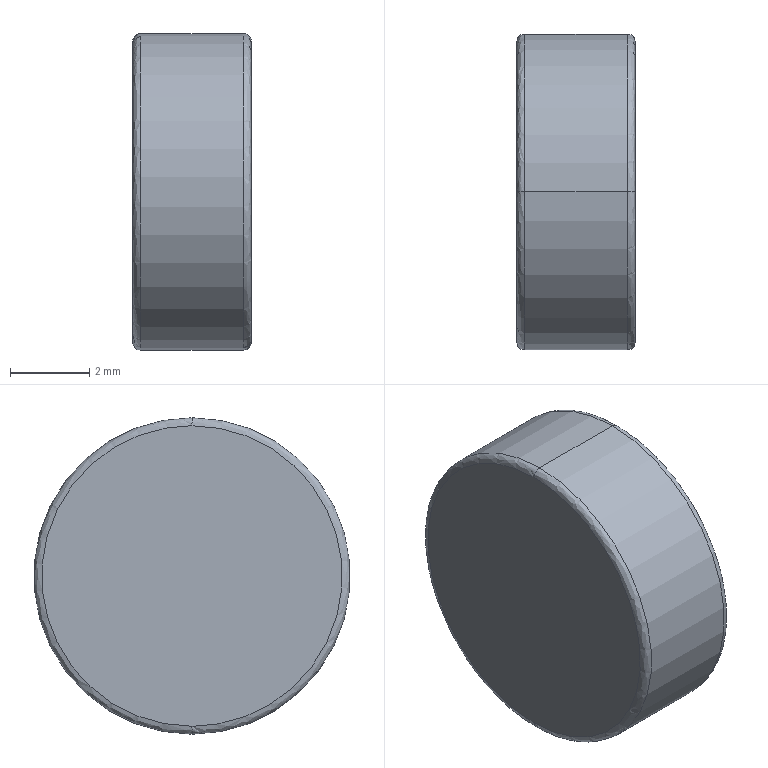Part | STEP file | Magnet dia 8 thickness 3 | 1 solid | 8 faces | box 3 x 8 x 8 mm | volume 150.376 mm3 | spline 4 | cylinder 2 | plane 2 | commonest cylinder face diameters 8 x2
STEP:
#1=CARTESIAN_POINT('',(0.,0.,0.));
#2=DIRECTION('',(0.,0.,1.));
#3=DIRECTION('',(1.,0.,0.));
#4=AXIS2_PLACEMENT_3D('',#1,#2,#3);
#5=CARTESIAN_POINT('',(2.8,0.,-4.));
#6=VERTEX_POINT('',#5);
#7=CARTESIAN_POINT('',(2.8,0.,4.));
#8=VERTEX_POINT('',#7);
#9=CARTESIAN_POINT('',(2.8,0.,0.));
#10=DIRECTION('',(1.,0.,0.));
#11=DIRECTION('',(0.,1.,0.));
#12=AXIS2_PLACEMENT_3D('',#9,#10,#11);
#13=CIRCLE('',#12,4.);
#14=CARTESIAN_POINT('',(2.8,0.,0.));
#15=DIRECTION('',(-1.,0.,0.));
#16=DIRECTION('',(0.,0.,1.));
#17=AXIS2_PLACEMENT_3D('',#14,#15,#16);
#18=CYLINDRICAL_SURFACE('',#17,4.);
#19=CARTESIAN_POINT('',(7.854,0.));
#20=DIRECTION('',(-1.,0.));
#21=VECTOR('',#20,1.);
#22=LINE('',#19,#21);
#23=(GEOMETRIC_REPRESENTATION_CONTEXT(2)PARAMETRIC_REPRESENTATION_CONTEXT()REPRESENTATION_CONTEXT('',''));
#24=DEFINITIONAL_REPRESENTATION('',(#22),#23);
#25=PCURVE('',#18,#24);
#26=CARTESIAN_POINT('',(2.999,0.,-3.78));
#27=CARTESIAN_POINT('',(2.999,7.56,-3.78));
#28=CARTESIAN_POINT('',(2.999,7.56,3.78));
#29=CARTESIAN_POINT('',(2.999,0.,3.78));
#30=CARTESIAN_POINT('',(3.013,0.,-3.916));
#31=CARTESIAN_POINT('',(3.013,7.832,-3.916));
#32=CARTESIAN_POINT('',(3.013,7.832,3.916));
#33=CARTESIAN_POINT('',(3.013,0.,3.916));
#34=CARTESIAN_POINT('',(2.916,0.,-4.013));
#35=CARTESIAN_POINT('',(2.916,8.025,-4.013));
#36=CARTESIAN_POINT('',(2.916,8.025,4.013));
#37=CARTESIAN_POINT('',(2.916,0.,4.013));
#38=CARTESIAN_POINT('',(2.78,0.,-3.999));
#39=CARTESIAN_POINT('',(2.78,7.998,-3.999));
#40=CARTESIAN_POINT('',(2.78,7.998,3.999));
#41=CARTESIAN_POINT('',(2.78,0.,3.999));
#42=(BOUNDED_SURFACE()B_SPLINE_SURFACE(3,3,((#26,#27,#28,#29),(#30,#31,#32,#33),(#34,#35,#36,#37),(#38,#39,#40,#41)),.UNSPECIFIED.,.F.,.F.,.F.)B_SPLINE_SURFACE_WITH_KNOTS((4,4),(4,4),(0.,1.),(0.,1.),.PIECEWISE_BEZIER_KNOTS.)GEOMETRIC_REPRESENTATION_ITEM()RATIONAL_B_SPLINE_SURFACE(((1.,0.3333,0.3333,1.),(0.7553,0.2518,0.2518,0.7553),(0.7553,0.2518,0.2518,0.7553),(1.,0.3333,0.3333,1.)))REPRESENTATION_ITEM('')SURFACE());
#43=CARTESIAN_POINT('',(0.9369,0.));
#44=CARTESIAN_POINT('',(0.9369,0.02375));
#45=CARTESIAN_POINT('',(0.9369,0.06805));
#46=CARTESIAN_POINT('',(0.9369,0.1267));
#47=CARTESIAN_POINT('',(0.9369,0.1794));
#48=CARTESIAN_POINT('',(0.9369,0.2276));
#49=CARTESIAN_POINT('',(0.9369,0.2721));
#50=CARTESIAN_POINT('',(0.9369,0.3139));
#51=CARTESIAN_POINT('',(0.9369,0.3535));
#52=CARTESIAN_POINT('',(0.9369,0.3914));
#53=CARTESIAN_POINT('',(0.9369,0.4282));
#54=CARTESIAN_POINT('',(0.9369,0.4643));
#55=CARTESIAN_POINT('',(0.9369,0.5));
#56=CARTESIAN_POINT('',(0.9369,0.5357));
#57=CARTESIAN_POINT('',(0.9369,0.5718));
#58=CARTESIAN_POINT('',(0.9369,0.6086));
#59=CARTESIAN_POINT('',(0.9369,0.6465));
#60=CARTESIAN_POINT('',(0.9369,0.6861));
#61=CARTESIAN_POINT('',(0.9369,0.7279));
#62=CARTESIAN_POINT('',(0.9369,0.7724));
#63=CARTESIAN_POINT('',(0.9369,0.8206));
#64=CARTESIAN_POINT('',(0.9369,0.8733));
#65=CARTESIAN_POINT('',(0.9369,0.9319));
#66=CARTESIAN_POINT('',(0.9369,0.9763));
#67=CARTESIAN_POINT('',(0.9369,1.));
#68=B_SPLINE_CURVE_WITH_KNOTS('',3,(#43,#44,#45,#46,#47,#48,#49,#50,#51,#52,#53,#54,#55,#56,#57,#58,#59,#60,#61,#62,#63,#64,#65,#66,#67),.UNSPECIFIED.,.F.,.F.,(4,1,1,1,1,1,1,1,1,1,1,1,1,1,1,1,1,1,1,1,1,1,4),(4.712,4.855,4.998,5.141,5.284,5.426,5.569,5.712,5.855,5.998,6.14,6.283,6.426,6.569,6.712,6.854,6.997,7.14,7.283,7.426,7.568,7.711,7.854),.QUASI_UNIFORM_KNOTS.);
#69=(GEOMETRIC_REPRESENTATION_CONTEXT(2)PARAMETRIC_REPRESENTATION_CONTEXT()REPRESENTATION_CONTEXT('',''));
#70=DEFINITIONAL_REPRESENTATION('',(#68),#69);
#71=PCURVE('',#42,#70);
#72=SURFACE_CURVE('',#13,(#25,#71),.PCURVE_S1.);
#73=EDGE_CURVE('',#6,#8,#72,.T.);
#74=ORIENTED_EDGE('',*,*,#73,.F.);
#75=CARTESIAN_POINT('',(0.2,0.,-4.));
#76=VERTEX_POINT('',#75);
#77=CARTESIAN_POINT('',(2.8,0.,-4.));
#78=DIRECTION('',(-1.,0.,0.));
#79=VECTOR('',#78,1.);
#80=LINE('',#77,#79);
#81=CARTESIAN_POINT('',(3.142,0.));
#82=DIRECTION('',(0.,1.));
#83=VECTOR('',#82,1.);
#84=LINE('',#81,#83);
#85=(GEOMETRIC_REPRESENTATION_CONTEXT(2)PARAMETRIC_REPRESENTATION_CONTEXT()REPRESENTATION_CONTEXT('',''));
#86=DEFINITIONAL_REPRESENTATION('',(#84),#85);
#87=PCURVE('',#18,#86);
#88=CARTESIAN_POINT('',(2.8,0.,0.));
#89=DIRECTION('',(-1.,0.,0.));
#90=DIRECTION('',(0.,0.,1.));
#91=AXIS2_PLACEMENT_3D('',#88,#89,#90);
#92=CYLINDRICAL_SURFACE('',#91,4.);
#93=CARTESIAN_POINT('',(3.142,0.));
#94=DIRECTION('',(0.,1.));
#95=VECTOR('',#94,1.);
#96=LINE('',#93,#95);
#97=(GEOMETRIC_REPRESENTATION_CONTEXT(2)PARAMETRIC_REPRESENTATION_CONTEXT()REPRESENTATION_CONTEXT('',''));
#98=DEFINITIONAL_REPRESENTATION('',(#96),#97);
#99=PCURVE('',#92,#98);
#100=SURFACE_CURVE('',#80,(#87,#99),.PCURVE_S1.);
#101=EDGE_CURVE('',#6,#76,#100,.T.);
#102=ORIENTED_EDGE('',*,*,#101,.T.);
#103=CARTESIAN_POINT('',(0.2,0.,4.));
#104=VERTEX_POINT('',#103);
#105=CARTESIAN_POINT('',(0.2,0.,0.));
#106=DIRECTION('',(-1.,0.,0.));
#107=DIRECTION('',(0.,0.,1.));
#108=AXIS2_PLACEMENT_3D('',#105,#106,#107);
#109=CIRCLE('',#108,4.);
#110=CARTESIAN_POINT('',(0.,2.6));
#111=DIRECTION('',(1.,0.));
#112=VECTOR('',#111,1.);
#113=LINE('',#110,#112);
#114=(GEOMETRIC_REPRESENTATION_CONTEXT(2)PARAMETRIC_REPRESENTATION_CONTEXT()REPRESENTATION_CONTEXT('',''));
#115=DEFINITIONAL_REPRESENTATION('',(#113),#114);
#116=PCURVE('',#18,#115);
#117=CARTESIAN_POINT('',(0.22,0.,-3.999));
#118=CARTESIAN_POINT('',(0.22,7.998,-3.999));
#119=CARTESIAN_POINT('',(0.22,7.998,3.999));
#120=CARTESIAN_POINT('',(0.22,0.,3.999));
#121=CARTESIAN_POINT('',(0.08399,0.,-4.013));
#122=CARTESIAN_POINT('',(0.08399,8.025,-4.013));
#123=CARTESIAN_POINT('',(0.08399,8.025,4.013));
#124=CARTESIAN_POINT('',(0.08399,0.,4.013));
#125=CARTESIAN_POINT('',(-0.01264,0.,-3.916));
#126=CARTESIAN_POINT('',(-0.01264,7.832,-3.916));
#127=CARTESIAN_POINT('',(-0.01264,7.832,3.916));
#128=CARTESIAN_POINT('',(-0.01264,0.,3.916));
#129=CARTESIAN_POINT('',(0.0009992,0.,-3.78));
#130=CARTESIAN_POINT('',(0.0009992,7.56,-3.78));
#131=CARTESIAN_POINT('',(0.0009992,7.56,3.78));
#132=CARTESIAN_POINT('',(0.0009992,0.,3.78));
#133=(BOUNDED_SURFACE()B_SPLINE_SURFACE(3,3,((#117,#118,#119,#120),(#121,#122,#123,#124),(#125,#126,#127,#128),(#129,#130,#131,#132)),.UNSPECIFIED.,.F.,.F.,.F.)B_SPLINE_SURFACE_WITH_KNOTS((4,4),(4,4),(0.,1.),(0.,1.),.PIECEWISE_BEZIER_KNOTS.)GEOMETRIC_REPRESENTATION_ITEM()RATIONAL_B_SPLINE_SURFACE(((1.,0.3333,0.3333,1.),(0.7553,0.2518,0.2518,0.7553),(0.7553,0.2518,0.2518,0.7553),(1.,0.3333,0.3333,1.)))REPRESENTATION_ITEM('')SURFACE());
#134=CARTESIAN_POINT('',(0.06314,1.));
#135=CARTESIAN_POINT('',(0.06314,0.9763));
#136=CARTESIAN_POINT('',(0.06314,0.9319));
#137=CARTESIAN_POINT('',(0.06314,0.8733));
#138=CARTESIAN_POINT('',(0.06314,0.8206));
#139=CARTESIAN_POINT('',(0.06314,0.7724));
#140=CARTESIAN_POINT('',(0.06314,0.7279));
#141=CARTESIAN_POINT('',(0.06314,0.6861));
#142=CARTESIAN_POINT('',(0.06314,0.6465));
#143=CARTESIAN_POINT('',(0.06314,0.6086));
#144=CARTESIAN_POINT('',(0.06314,0.5718));
#145=CARTESIAN_POINT('',(0.06314,0.5357));
#146=CARTESIAN_POINT('',(0.06314,0.5));
#147=CARTESIAN_POINT('',(0.06314,0.4643));
#148=CARTESIAN_POINT('',(0.06314,0.4282));
#149=CARTESIAN_POINT('',(0.06314,0.3914));
#150=CARTESIAN_POINT('',(0.06314,0.3535));
#151=CARTESIAN_POINT('',(0.06314,0.3139));
#152=CARTESIAN_POINT('',(0.06314,0.2721));
#153=CARTESIAN_POINT('',(0.06314,0.2276));
#154=CARTESIAN_POINT('',(0.06314,0.1794));
#155=CARTESIAN_POINT('',(0.06314,0.1267));
#156=CARTESIAN_POINT('',(0.06314,0.06805));
#157=CARTESIAN_POINT('',(0.06314,0.02375));
#158=CARTESIAN_POINT('',(0.06314,0.));
#159=B_SPLINE_CURVE_WITH_KNOTS('',3,(#134,#135,#136,#137,#138,#139,#140,#141,#142,#143,#144,#145,#146,#147,#148,#149,#150,#151,#152,#153,#154,#155,#156,#157,#158),.UNSPECIFIED.,.F.,.F.,(4,1,1,1,1,1,1,1,1,1,1,1,1,1,1,1,1,1,1,1,1,1,4),(0.,0.1428,0.2856,0.4284,0.5712,0.714,0.8568,0.9996,1.142,1.285,1.428,1.571,1.714,1.856,1.999,2.142,2.285,2.428,2.57,2.713,2.856,2.999,3.142),.QUASI_UNIFORM_KNOTS.);
#160=(GEOMETRIC_REPRESENTATION_CONTEXT(2)PARAMETRIC_REPRESENTATION_CONTEXT()REPRESENTATION_CONTEXT('',''));
#161=DEFINITIONAL_REPRESENTATION('',(#159),#160);
#162=PCURVE('',#133,#161);
#163=SURFACE_CURVE('',#109,(#116,#162),.PCURVE_S1.);
#164=EDGE_CURVE('',#104,#76,#163,.T.);
#165=ORIENTED_EDGE('',*,*,#164,.F.);
#166=CARTESIAN_POINT('',(2.8,0.,4.));
#167=DIRECTION('',(-1.,0.,0.));
#168=VECTOR('',#167,1.);
#169=LINE('',#166,#168);
#170=CARTESIAN_POINT('',(0.,0.));
#171=DIRECTION('',(0.,1.));
#172=VECTOR('',#171,1.);
#173=LINE('',#170,#172);
#174=(GEOMETRIC_REPRESENTATION_CONTEXT(2)PARAMETRIC_REPRESENTATION_CONTEXT()REPRESENTATION_CONTEXT('',''));
#175=DEFINITIONAL_REPRESENTATION('',(#173),#174);
#176=PCURVE('',#18,#175);
#177=CARTESIAN_POINT('',(6.283,0.));
#178=DIRECTION('',(0.,1.));
#179=VECTOR('',#178,1.);
#180=LINE('',#177,#179);
#181=(GEOMETRIC_REPRESENTATION_CONTEXT(2)PARAMETRIC_REPRESENTATION_CONTEXT()REPRESENTATION_CONTEXT('',''));
#182=DEFINITIONAL_REPRESENTATION('',(#180),#181);
#183=PCURVE('',#92,#182);
#184=SURFACE_CURVE('',#169,(#176,#183),.PCURVE_S1.);
#185=EDGE_CURVE('',#8,#104,#184,.T.);
#186=ORIENTED_EDGE('',*,*,#185,.F.);
#187=EDGE_LOOP('',(#74,#102,#165,#186));
#188=FACE_BOUND('',#187,.T.);
#189=ADVANCED_FACE('',(#188),#18,.T.);
#190=CARTESIAN_POINT('',(3.,0.,3.8));
#191=VERTEX_POINT('',#190);
#192=CARTESIAN_POINT('',(3.,0.,-3.8));
#193=VERTEX_POINT('',#192);
#194=CARTESIAN_POINT('',(3.,0.,3.8));
#195=CARTESIAN_POINT('',(3.,7.6,3.8));
#196=CARTESIAN_POINT('',(3.,7.6,-3.8));
#197=CARTESIAN_POINT('',(3.,0.,-3.8));
#198=(BOUNDED_CURVE()B_SPLINE_CURVE(3,(#194,#195,#196,#197),.UNSPECIFIED.,.F.,.F.)B_SPLINE_CURVE_WITH_KNOTS((4,4),(0.,1.),.PIECEWISE_BEZIER_KNOTS.)CURVE()GEOMETRIC_REPRESENTATION_ITEM()RATIONAL_B_SPLINE_CURVE((0.9566,0.3189,0.3189,0.9566))REPRESENTATION_ITEM(''));
#199=CARTESIAN_POINT('',(0.06314,1.));
#200=DIRECTION('',(0.,-1.));
#201=VECTOR('',#200,1.);
#202=LINE('',#199,#201);
#203=(GEOMETRIC_REPRESENTATION_CONTEXT(2)PARAMETRIC_REPRESENTATION_CONTEXT()REPRESENTATION_CONTEXT('',''));
#204=DEFINITIONAL_REPRESENTATION('',(#202),#203);
#205=PCURVE('',#42,#204);
#206=CARTESIAN_POINT('',(3.,-3.846,3.846));
#207=DIRECTION('',(1.,0.,0.));
#208=DIRECTION('',(0.,0.,-1.));
#209=AXIS2_PLACEMENT_3D('',#206,#207,#208);
#210=PLANE('',#209);
#211=CARTESIAN_POINT('',(0.0456,3.846));
#212=CARTESIAN_POINT('',(0.0456,11.446));
#213=CARTESIAN_POINT('',(7.646,11.446));
#214=CARTESIAN_POINT('',(7.646,3.846));
#215=(BOUNDED_CURVE()B_SPLINE_CURVE(3,(#211,#212,#213,#214),.UNSPECIFIED.,.F.,.F.)B_SPLINE_CURVE_WITH_KNOTS((4,4),(0.,1.),.PIECEWISE_BEZIER_KNOTS.)CURVE()GEOMETRIC_REPRESENTATION_ITEM()RATIONAL_B_SPLINE_CURVE((0.9566,0.3189,0.3189,0.9566))REPRESENTATION_ITEM(''));
#216=(GEOMETRIC_REPRESENTATION_CONTEXT(2)PARAMETRIC_REPRESENTATION_CONTEXT()REPRESENTATION_CONTEXT('',''));
#217=DEFINITIONAL_REPRESENTATION('',(#215),#216);
#218=PCURVE('',#210,#217);
#219=SURFACE_CURVE('',#198,(#205,#218),.PCURVE_S1.);
#220=EDGE_CURVE('',#191,#193,#219,.T.);
#221=ORIENTED_EDGE('',*,*,#220,.T.);
#222=CARTESIAN_POINT('',(2.8,0.,-4.));
#223=CARTESIAN_POINT('',(2.917,0.,-4.));
#224=CARTESIAN_POINT('',(3.,0.,-3.917));
#225=CARTESIAN_POINT('',(3.,0.,-3.8));
#226=(BOUNDED_CURVE()B_SPLINE_CURVE(3,(#222,#223,#224,#225),.UNSPECIFIED.,.F.,.F.)B_SPLINE_CURVE_WITH_KNOTS((4,4),(0.06314,0.9369),.PIECEWISE_BEZIER_KNOTS.)CURVE()GEOMETRIC_REPRESENTATION_ITEM()RATIONAL_B_SPLINE_CURVE((0.9566,0.7698,0.7698,0.9566))REPRESENTATION_ITEM(''));
#227=CARTESIAN_POINT('',(0.9369,0.));
#228=CARTESIAN_POINT('',(0.06314,0.));
#229=B_SPLINE_CURVE_WITH_KNOTS('',1,(#227,#228),.UNSPECIFIED.,.F.,.F.,(2,2),(0.06314,0.9369),.PIECEWISE_BEZIER_KNOTS.);
#230=(GEOMETRIC_REPRESENTATION_CONTEXT(2)PARAMETRIC_REPRESENTATION_CONTEXT()REPRESENTATION_CONTEXT('',''));
#231=DEFINITIONAL_REPRESENTATION('',(#229),#230);
#232=PCURVE('',#42,#231);
#233=CARTESIAN_POINT('',(2.999,0.,3.78));
#234=CARTESIAN_POINT('',(2.999,-7.56,3.78));
#235=CARTESIAN_POINT('',(2.999,-7.56,-3.78));
#236=CARTESIAN_POINT('',(2.999,0.,-3.78));
#237=CARTESIAN_POINT('',(3.013,0.,3.916));
#238=CARTESIAN_POINT('',(3.013,-7.832,3.916));
#239=CARTESIAN_POINT('',(3.013,-7.832,-3.916));
#240=CARTESIAN_POINT('',(3.013,0.,-3.916));
#241=CARTESIAN_POINT('',(2.916,0.,4.013));
#242=CARTESIAN_POINT('',(2.916,-8.025,4.013));
#243=CARTESIAN_POINT('',(2.916,-8.025,-4.013));
#244=CARTESIAN_POINT('',(2.916,0.,-4.013));
#245=CARTESIAN_POINT('',(2.78,0.,3.999));
#246=CARTESIAN_POINT('',(2.78,-7.998,3.999));
#247=CARTESIAN_POINT('',(2.78,-7.998,-3.999));
#248=CARTESIAN_POINT('',(2.78,0.,-3.999));
#249=(BOUNDED_SURFACE()B_SPLINE_SURFACE(3,3,((#233,#234,#235,#236),(#237,#238,#239,#240),(#241,#242,#243,#244),(#245,#246,#247,#248)),.UNSPECIFIED.,.F.,.F.,.F.)B_SPLINE_SURFACE_WITH_KNOTS((4,4),(4,4),(0.,1.),(0.,1.),.PIECEWISE_BEZIER_KNOTS.)GEOMETRIC_REPRESENTATION_ITEM()RATIONAL_B_SPLINE_SURFACE(((1.,0.3333,0.3333,1.),(0.7553,0.2518,0.2518,0.7553),(0.7553,0.2518,0.2518,0.7553),(1.,0.3333,0.3333,1.)))REPRESENTATION_ITEM('')SURFACE());
#250=CARTESIAN_POINT('',(0.9369,1.));
#251=CARTESIAN_POINT('',(0.06314,1.));
#252=B_SPLINE_CURVE_WITH_KNOTS('',1,(#250,#251),.UNSPECIFIED.,.F.,.F.,(2,2),(0.06314,0.9369),.PIECEWISE_BEZIER_KNOTS.);
#253=(GEOMETRIC_REPRESENTATION_CONTEXT(2)PARAMETRIC_REPRESENTATION_CONTEXT()REPRESENTATION_CONTEXT('',''));
#254=DEFINITIONAL_REPRESENTATION('',(#252),#253);
#255=PCURVE('',#249,#254);
#256=SURFACE_CURVE('',#226,(#232,#255),.PCURVE_S1.);
#257=EDGE_CURVE('',#6,#193,#256,.T.);
#258=ORIENTED_EDGE('',*,*,#257,.F.);
#259=ORIENTED_EDGE('',*,*,#73,.T.);
#260=CARTESIAN_POINT('',(3.,0.,3.8));
#261=CARTESIAN_POINT('',(3.,0.,3.917));
#262=CARTESIAN_POINT('',(2.917,0.,4.));
#263=CARTESIAN_POINT('',(2.8,0.,4.));
#264=(BOUNDED_CURVE()B_SPLINE_CURVE(3,(#260,#261,#262,#263),.UNSPECIFIED.,.F.,.F.)B_SPLINE_CURVE_WITH_KNOTS((4,4),(0.06314,0.9369),.PIECEWISE_BEZIER_KNOTS.)CURVE()GEOMETRIC_REPRESENTATION_ITEM()RATIONAL_B_SPLINE_CURVE((0.9566,0.7698,0.7698,0.9566))REPRESENTATION_ITEM(''));
#265=CARTESIAN_POINT('',(0.06314,1.));
#266=CARTESIAN_POINT('',(0.9369,1.));
#267=B_SPLINE_CURVE_WITH_KNOTS('',1,(#265,#266),.UNSPECIFIED.,.F.,.F.,(2,2),(0.06314,0.9369),.PIECEWISE_BEZIER_KNOTS.);
#268=(GEOMETRIC_REPRESENTATION_CONTEXT(2)PARAMETRIC_REPRESENTATION_CONTEXT()REPRESENTATION_CONTEXT('',''));
#269=DEFINITIONAL_REPRESENTATION('',(#267),#268);
#270=PCURVE('',#42,#269);
#271=CARTESIAN_POINT('',(0.06314,0.));
#272=CARTESIAN_POINT('',(0.9369,0.));
#273=B_SPLINE_CURVE_WITH_KNOTS('',1,(#271,#272),.UNSPECIFIED.,.F.,.F.,(2,2),(0.06314,0.9369),.PIECEWISE_BEZIER_KNOTS.);
#274=(GEOMETRIC_REPRESENTATION_CONTEXT(2)PARAMETRIC_REPRESENTATION_CONTEXT()REPRESENTATION_CONTEXT('',''));
#275=DEFINITIONAL_REPRESENTATION('',(#273),#274);
#276=PCURVE('',#249,#275);
#277=SURFACE_CURVE('',#264,(#270,#276),.PCURVE_S1.);
#278=EDGE_CURVE('',#191,#8,#277,.T.);
#279=ORIENTED_EDGE('',*,*,#278,.F.);
#280=EDGE_LOOP('',(#221,#258,#259,#279));
#281=FACE_BOUND('',#280,.T.);
#282=ADVANCED_FACE('',(#281),#42,.T.);
#283=ORIENTED_EDGE('',*,*,#220,.F.);
#284=CARTESIAN_POINT('',(3.,0.,3.8));
#285=CARTESIAN_POINT('',(3.,-0.1809,3.8));
#286=CARTESIAN_POINT('',(3.,-0.4495,3.781));
#287=CARTESIAN_POINT('',(3.,-0.7583,3.726));
#288=CARTESIAN_POINT('',(3.,-0.9115,3.69));
#289=CARTESIAN_POINT('',(3.,-0.9879,3.669));
#290=CARTESIAN_POINT('',(3.,-1.021,3.66));
#291=CARTESIAN_POINT('',(3.,-1.042,3.654));
#292=CARTESIAN_POINT('',(3.,-1.051,3.652));
#293=CARTESIAN_POINT('',(3.,-1.167,3.618));
#294=CARTESIAN_POINT('',(3.,-1.32,3.566));
#295=CARTESIAN_POINT('',(3.,-1.494,3.495));
#296=CARTESIAN_POINT('',(3.,-1.58,3.456));
#297=CARTESIAN_POINT('',(3.,-1.617,3.439));
#298=CARTESIAN_POINT('',(3.,-1.641,3.427));
#299=CARTESIAN_POINT('',(3.,-1.652,3.422));
#300=CARTESIAN_POINT('',(3.,-1.773,3.363));
#301=CARTESIAN_POINT('',(3.,-1.932,3.276));
#302=CARTESIAN_POINT('',(3.,-2.108,3.163));
#303=CARTESIAN_POINT('',(3.,-2.195,3.102));
#304=CARTESIAN_POINT('',(3.,-2.231,3.076));
#305=CARTESIAN_POINT('',(3.,-2.256,3.058));
#306=CARTESIAN_POINT('',(3.,-2.267,3.05));
#307=CARTESIAN_POINT('',(3.,-2.387,2.96));
#308=CARTESIAN_POINT('',(3.,-2.539,2.833));
#309=CARTESIAN_POINT('',(3.,-2.705,2.67));
#310=CARTESIAN_POINT('',(3.,-2.785,2.586));
#311=CARTESIAN_POINT('',(3.,-2.819,2.549));
#312=CARTESIAN_POINT('',(3.,-2.841,2.524));
#313=CARTESIAN_POINT('',(3.,-2.851,2.512));
#314=CARTESIAN_POINT('',(3.,-2.958,2.39));
#315=CARTESIAN_POINT('',(3.,-3.091,2.219));
#316=CARTESIAN_POINT('',(3.,-3.228,2.008));
#317=CARTESIAN_POINT('',(3.,-3.283,1.915));
#318=CARTESIAN_POINT('',(3.,-3.318,1.852));
#319=CARTESIAN_POINT('',(3.,-3.335,1.822));
#320=CARTESIAN_POINT('',(3.,-3.425,1.653));
#321=CARTESIAN_POINT('',(3.,-3.521,1.445));
#322=CARTESIAN_POINT('',(3.,-3.597,1.229));
#323=CARTESIAN_POINT('',(3.,-3.643,1.084));
#324=CARTESIAN_POINT('',(3.,-3.664,1.012));
#325=CARTESIAN_POINT('',(3.,-3.761,0.6288));
#326=CARTESIAN_POINT('',(3.,-3.8,0.3163));
#327=CARTESIAN_POINT('',(3.,-3.8,-0.1582));
#328=CARTESIAN_POINT('',(3.,-3.785,-0.3937));
#329=CARTESIAN_POINT('',(3.,-3.743,-0.6655));
#330=CARTESIAN_POINT('',(3.,-3.719,-0.7814));
#331=CARTESIAN_POINT('',(3.,-3.702,-0.8585));
#332=CARTESIAN_POINT('',(3.,-3.693,-0.8982));
#333=CARTESIAN_POINT('',(3.,-3.645,-1.084));
#334=CARTESIAN_POINT('',(3.,-3.576,-1.302));
#335=CARTESIAN_POINT('',(3.,-3.472,-1.548));
#336=CARTESIAN_POINT('',(3.,-3.414,-1.669));
#337=CARTESIAN_POINT('',(3.,-3.388,-1.72));
#338=CARTESIAN_POINT('',(3.,-3.371,-1.754));
#339=CARTESIAN_POINT('',(3.,-3.361,-1.772));
#340=CARTESIAN_POINT('',(3.,-3.285,-1.916));
#341=CARTESIAN_POINT('',(3.,-3.173,-2.1));
#342=CARTESIAN_POINT('',(3.,-3.024,-2.303));
#343=CARTESIAN_POINT('',(3.,-2.945,-2.402));
#344=CARTESIAN_POINT('',(3.,-2.91,-2.444));
#345=CARTESIAN_POINT('',(3.,-2.887,-2.471));
#346=CARTESIAN_POINT('',(3.,-2.874,-2.486));
#347=CARTESIAN_POINT('',(3.,-2.775,-2.599));
#348=CARTESIAN_POINT('',(3.,-2.637,-2.742));
#349=CARTESIAN_POINT('',(3.,-2.463,-2.895));
#350=CARTESIAN_POINT('',(3.,-2.372,-2.969));
#351=CARTESIAN_POINT('',(3.,-2.333,-3.));
#352=CARTESIAN_POINT('',(3.,-2.307,-3.02));
#353=CARTESIAN_POINT('',(3.,-2.292,-3.031));
#354=CARTESIAN_POINT('',(3.,-2.184,-3.112));
#355=CARTESIAN_POINT('',(3.,-2.035,-3.213));
#356=CARTESIAN_POINT('',(3.,-1.853,-3.319));
#357=CARTESIAN_POINT('',(3.,-1.76,-3.368));
#358=CARTESIAN_POINT('',(3.,-1.719,-3.389));
#359=CARTESIAN_POINT('',(3.,-1.692,-3.402));
#360=CARTESIAN_POINT('',(3.,-1.677,-3.41));
#361=CARTESIAN_POINT('',(3.,-1.568,-3.463));
#362=CARTESIAN_POINT('',(3.,-1.421,-3.527));
#363=CARTESIAN_POINT('',(3.,-1.244,-3.591));
#364=CARTESIAN_POINT('',(3.,-1.154,-3.621));
#365=CARTESIAN_POINT('',(3.,-1.116,-3.633));
#366=CARTESIAN_POINT('',(3.,-1.09,-3.64));
#367=CARTESIAN_POINT('',(3.,-1.075,-3.645));
#368=CARTESIAN_POINT('',(3.,-0.9724,-3.675));
#369=CARTESIAN_POINT('',(3.,-0.8337,-3.71));
#370=CARTESIAN_POINT('',(3.,-0.6698,-3.741));
#371=CARTESIAN_POINT('',(3.,-0.5873,-3.754));
#372=CARTESIAN_POINT('',(3.,-0.5518,-3.76));
#373=CARTESIAN_POINT('',(3.,-0.5281,-3.763));
#374=CARTESIAN_POINT('',(3.,-0.5149,-3.765));
#375=CARTESIAN_POINT('',(3.,-0.3372,-3.789));
#376=CARTESIAN_POINT('',(3.,-0.1691,-3.8));
#377=CARTESIAN_POINT('',(3.,0.,-3.8));
#378=B_SPLINE_CURVE_WITH_KNOTS('',3,(#284,#285,#286,#287,#288,#289,#290,#291,#292,#293,#294,#295,#296,#297,#298,#299,#300,#301,#302,#303,#304,#305,#306,#307,#308,#309,#310,#311,#312,#313,#314,#315,#316,#317,#318,#319,#320,#321,#322,#323,#324,#325,#326,#327,#328,#329,#330,#331,#332,#333,#334,#335,#336,#337,#338,#339,#340,#341,#342,#343,#344,#345,#346,#347,#348,#349,#350,#351,#352,#353,#354,#355,#356,#357,#358,#359,#360,#361,#362,#363,#364,#365,#366,#367,#368,#369,#370,#371,#372,#373,#374,#375,#376,#377),.UNSPECIFIED.,.F.,.F.,(4,1,1,1,1,2,2,1,1,1,2,2,1,1,1,2,2,1,1,1,2,2,1,1,2,2,1,2,2,2,1,1,2,2,1,1,1,2,2,1,1,1,2,2,1,1,1,2,2,1,1,1,2,2,1,1,1,2,2,1,1,1,2,2,4),(0.,0.0625,0.09375,0.1094,0.1172,0.1211,0.125,0.1562,0.1719,0.1797,0.1836,0.1875,0.2188,0.2344,0.2422,0.2461,0.25,0.2812,0.2969,0.3047,0.3086,0.3125,0.3438,0.3594,0.3672,0.375,0.4062,0.4219,0.4375,0.5,0.5312,0.5469,0.5547,0.5625,0.5938,0.6094,0.6172,0.6211,0.625,0.6562,0.6719,0.6797,0.6836,0.6875,0.7188,0.7344,0.7422,0.7461,0.75,0.7812,0.7969,0.8047,0.8086,0.8125,0.8438,0.8594,0.8672,0.8711,0.875,0.9062,0.9219,0.9297,0.9336,0.9375,1.),.UNSPECIFIED.);
#379=CARTESIAN_POINT('',(0.0456,3.846));
#380=CARTESIAN_POINT('',(0.0456,3.665));
#381=CARTESIAN_POINT('',(0.0646,3.396));
#382=CARTESIAN_POINT('',(0.12,3.087));
#383=CARTESIAN_POINT('',(0.156,2.934));
#384=CARTESIAN_POINT('',(0.1761,2.858));
#385=CARTESIAN_POINT('',(0.1852,2.825));
#386=CARTESIAN_POINT('',(0.1913,2.803));
#387=CARTESIAN_POINT('',(0.1938,2.795));
#388=CARTESIAN_POINT('',(0.2277,2.678));
#389=CARTESIAN_POINT('',(0.2793,2.526));
#390=CARTESIAN_POINT('',(0.3509,2.352));
#391=CARTESIAN_POINT('',(0.3894,2.266));
#392=CARTESIAN_POINT('',(0.4066,2.229));
#393=CARTESIAN_POINT('',(0.4181,2.205));
#394=CARTESIAN_POINT('',(0.4233,2.194));
#395=CARTESIAN_POINT('',(0.4826,2.072));
#396=CARTESIAN_POINT('',(0.5692,1.914));
#397=CARTESIAN_POINT('',(0.6831,1.737));
#398=CARTESIAN_POINT('',(0.7433,1.651));
#399=CARTESIAN_POINT('',(0.7697,1.614));
#400=CARTESIAN_POINT('',(0.7876,1.59));
#401=CARTESIAN_POINT('',(0.7956,1.579));
#402=CARTESIAN_POINT('',(0.8855,1.459));
#403=CARTESIAN_POINT('',(1.013,1.306));
#404=CARTESIAN_POINT('',(1.175,1.14));
#405=CARTESIAN_POINT('',(1.26,1.06));
#406=CARTESIAN_POINT('',(1.297,1.027));
#407=CARTESIAN_POINT('',(1.322,1.005));
#408=CARTESIAN_POINT('',(1.333,0.9945));
#409=CARTESIAN_POINT('',(1.456,0.8875));
#410=CARTESIAN_POINT('',(1.626,0.7549));
#411=CARTESIAN_POINT('',(1.838,0.6179));
#412=CARTESIAN_POINT('',(1.931,0.563));
#413=CARTESIAN_POINT('',(1.994,0.5272));
#414=CARTESIAN_POINT('',(2.024,0.5107));
#415=CARTESIAN_POINT('',(2.193,0.4205));
#416=CARTESIAN_POINT('',(2.401,0.3251));
#417=CARTESIAN_POINT('',(2.617,0.249));
#418=CARTESIAN_POINT('',(2.762,0.2025));
#419=CARTESIAN_POINT('',(2.834,0.182));
#420=CARTESIAN_POINT('',(3.217,0.08462));
#421=CARTESIAN_POINT('',(3.529,0.04565));
#422=CARTESIAN_POINT('',(4.004,0.04558));
#423=CARTESIAN_POINT('',(4.239,0.06018));
#424=CARTESIAN_POINT('',(4.511,0.1028));
#425=CARTESIAN_POINT('',(4.627,0.1266));
#426=CARTESIAN_POINT('',(4.704,0.1436));
#427=CARTESIAN_POINT('',(4.744,0.1531));
#428=CARTESIAN_POINT('',(4.93,0.2003));
#429=CARTESIAN_POINT('',(5.148,0.2698));
#430=CARTESIAN_POINT('',(5.394,0.3737));
#431=CARTESIAN_POINT('',(5.514,0.4313));
#432=CARTESIAN_POINT('',(5.566,0.4572));
#433=CARTESIAN_POINT('',(5.6,0.4747));
#434=CARTESIAN_POINT('',(5.618,0.4842));
#435=CARTESIAN_POINT('',(5.761,0.5607));
#436=CARTESIAN_POINT('',(5.946,0.6729));
#437=CARTESIAN_POINT('',(6.149,0.8218));
#438=CARTESIAN_POINT('',(6.248,0.9007));
#439=CARTESIAN_POINT('',(6.289,0.9355));
#440=CARTESIAN_POINT('',(6.317,0.9589));
#441=CARTESIAN_POINT('',(6.332,0.9716));
#442=CARTESIAN_POINT('',(6.445,1.07));
#443=CARTESIAN_POINT('',(6.587,1.209));
#444=CARTESIAN_POINT('',(6.741,1.383));
#445=CARTESIAN_POINT('',(6.814,1.473));
#446=CARTESIAN_POINT('',(6.845,1.513));
#447=CARTESIAN_POINT('',(6.865,1.539));
#448=CARTESIAN_POINT('',(6.877,1.554));
#449=CARTESIAN_POINT('',(6.958,1.662));
#450=CARTESIAN_POINT('',(7.059,1.811));
#451=CARTESIAN_POINT('',(7.164,1.993));
#452=CARTESIAN_POINT('',(7.214,2.086));
#453=CARTESIAN_POINT('',(7.234,2.126));
#454=CARTESIAN_POINT('',(7.248,2.153));
#455=CARTESIAN_POINT('',(7.255,2.168));
#456=CARTESIAN_POINT('',(7.309,2.277));
#457=CARTESIAN_POINT('',(7.373,2.425));
#458=CARTESIAN_POINT('',(7.437,2.602));
#459=CARTESIAN_POINT('',(7.466,2.691));
#460=CARTESIAN_POINT('',(7.478,2.73));
#461=CARTESIAN_POINT('',(7.486,2.756));
#462=CARTESIAN_POINT('',(7.49,2.77));
#463=CARTESIAN_POINT('',(7.52,2.873));
#464=CARTESIAN_POINT('',(7.555,3.012));
#465=CARTESIAN_POINT('',(7.587,3.176));
#466=CARTESIAN_POINT('',(7.6,3.258));
#467=CARTESIAN_POINT('',(7.605,3.294));
#468=CARTESIAN_POINT('',(7.609,3.317));
#469=CARTESIAN_POINT('',(7.611,3.331));
#470=CARTESIAN_POINT('',(7.634,3.508));
#471=CARTESIAN_POINT('',(7.646,3.677));
#472=CARTESIAN_POINT('',(7.646,3.846));
#473=B_SPLINE_CURVE_WITH_KNOTS('',3,(#379,#380,#381,#382,#383,#384,#385,#386,#387,#388,#389,#390,#391,#392,#393,#394,#395,#396,#397,#398,#399,#400,#401,#402,#403,#404,#405,#406,#407,#408,#409,#410,#411,#412,#413,#414,#415,#416,#417,#418,#419,#420,#421,#422,#423,#424,#425,#426,#427,#428,#429,#430,#431,#432,#433,#434,#435,#436,#437,#438,#439,#440,#441,#442,#443,#444,#445,#446,#447,#448,#449,#450,#451,#452,#453,#454,#455,#456,#457,#458,#459,#460,#461,#462,#463,#464,#465,#466,#467,#468,#469,#470,#471,#472),.UNSPECIFIED.,.F.,.F.,(4,1,1,1,1,2,2,1,1,1,2,2,1,1,1,2,2,1,1,1,2,2,1,1,2,2,1,2,2,2,1,1,2,2,1,1,1,2,2,1,1,1,2,2,1,1,1,2,2,1,1,1,2,2,1,1,1,2,2,1,1,1,2,2,4),(0.,0.0625,0.09375,0.1094,0.1172,0.1211,0.125,0.1562,0.1719,0.1797,0.1836,0.1875,0.2188,0.2344,0.2422,0.2461,0.25,0.2812,0.2969,0.3047,0.3086,0.3125,0.3438,0.3594,0.3672,0.375,0.4062,0.4219,0.4375,0.5,0.5312,0.5469,0.5547,0.5625,0.5938,0.6094,0.6172,0.6211,0.625,0.6562,0.6719,0.6797,0.6836,0.6875,0.7188,0.7344,0.7422,0.7461,0.75,0.7812,0.7969,0.8047,0.8086,0.8125,0.8438,0.8594,0.8672,0.8711,0.875,0.9062,0.9219,0.9297,0.9336,0.9375,1.),.UNSPECIFIED.);
#474=(GEOMETRIC_REPRESENTATION_CONTEXT(2)PARAMETRIC_REPRESENTATION_CONTEXT()REPRESENTATION_CONTEXT('',''));
#475=DEFINITIONAL_REPRESENTATION('',(#473),#474);
#476=PCURVE('',#210,#475);
#477=CARTESIAN_POINT('',(0.06314,0.));
#478=CARTESIAN_POINT('',(0.06314,0.001442));
#479=CARTESIAN_POINT('',(0.06315,0.004313));
#480=CARTESIAN_POINT('',(0.06317,0.008577));
#481=CARTESIAN_POINT('',(0.0632,0.0128));
#482=CARTESIAN_POINT('',(0.06324,0.01698));
#483=CARTESIAN_POINT('',(0.06329,0.02113));
#484=CARTESIAN_POINT('',(0.06334,0.02524));
#485=CARTESIAN_POINT('',(0.06339,0.02931));
#486=CARTESIAN_POINT('',(0.06344,0.03335));
#487=CARTESIAN_POINT('',(0.06349,0.03735));
#488=CARTESIAN_POINT('',(0.06354,0.04132));
#489=CARTESIAN_POINT('',(0.06358,0.04525));
#490=CARTESIAN_POINT('',(0.06362,0.04915));
#491=CARTESIAN_POINT('',(0.06365,0.05303));
#492=CARTESIAN_POINT('',(0.06367,0.05687));
#493=CARTESIAN_POINT('',(0.06368,0.06068));
#494=CARTESIAN_POINT('',(0.06369,0.06446));
#495=CARTESIAN_POINT('',(0.06368,0.06822));
#496=CARTESIAN_POINT('',(0.06367,0.07194));
#497=CARTESIAN_POINT('',(0.06365,0.07564));
#498=CARTESIAN_POINT('',(0.06362,0.07932));
#499=CARTESIAN_POINT('',(0.06359,0.08297));
#500=CARTESIAN_POINT('',(0.06355,0.08659));
#501=CARTESIAN_POINT('',(0.0635,0.09019));
#502=CARTESIAN_POINT('',(0.06345,0.09377));
#503=CARTESIAN_POINT('',(0.0634,0.09732));
#504=CARTESIAN_POINT('',(0.06335,0.1009));
#505=CARTESIAN_POINT('',(0.0633,0.1044));
#506=CARTESIAN_POINT('',(0.06325,0.1079));
#507=CARTESIAN_POINT('',(0.06321,0.1113));
#508=CARTESIAN_POINT('',(0.06317,0.1148));
#509=CARTESIAN_POINT('',(0.06315,0.1182));
#510=CARTESIAN_POINT('',(0.06313,0.1217));
#511=CARTESIAN_POINT('',(0.06314,0.1248));
#512=CARTESIAN_POINT('',(0.06316,0.1291));
#513=CARTESIAN_POINT('',(0.06318,0.133));
#514=CARTESIAN_POINT('',(0.06319,0.1369));
#515=CARTESIAN_POINT('',(0.06321,0.1408));
#516=CARTESIAN_POINT('',(0.06322,0.1447));
#517=CARTESIAN_POINT('',(0.06323,0.1486));
#518=CARTESIAN_POINT('',(0.06323,0.1524));
#519=CARTESIAN_POINT('',(0.06322,0.1562));
#520=CARTESIAN_POINT('',(0.06321,0.16));
#521=CARTESIAN_POINT('',(0.0632,0.1637));
#522=CARTESIAN_POINT('',(0.06318,0.1674));
#523=CARTESIAN_POINT('',(0.06317,0.1711));
#524=CARTESIAN_POINT('',(0.06315,0.1748));
#525=CARTESIAN_POINT('',(0.06314,0.1785));
#526=CARTESIAN_POINT('',(0.06313,0.1821));
#527=CARTESIAN_POINT('',(0.06315,0.1856));
#528=CARTESIAN_POINT('',(0.06315,0.1895));
#529=CARTESIAN_POINT('',(0.06318,0.1935));
#530=CARTESIAN_POINT('',(0.0632,0.1974));
#531=CARTESIAN_POINT('',(0.06322,0.2013));
#532=CARTESIAN_POINT('',(0.06324,0.2052));
#533=CARTESIAN_POINT('',(0.06326,0.2091));
#534=CARTESIAN_POINT('',(0.06327,0.2129));
#535=CARTESIAN_POINT('',(0.06327,0.2167));
#536=CARTESIAN_POINT('',(0.06326,0.2205));
#537=CARTESIAN_POINT('',(0.06324,0.2243));
#538=CARTESIAN_POINT('',(0.06322,0.228));
#539=CARTESIAN_POINT('',(0.0632,0.2317));
#540=CARTESIAN_POINT('',(0.06318,0.2354));
#541=CARTESIAN_POINT('',(0.06315,0.2391));
#542=CARTESIAN_POINT('',(0.06314,0.2427));
#543=CARTESIAN_POINT('',(0.06313,0.2464));
#544=CARTESIAN_POINT('',(0.06314,0.2499));
#545=CARTESIAN_POINT('',(0.06317,0.254));
#546=CARTESIAN_POINT('',(0.0632,0.2579));
#547=CARTESIAN_POINT('',(0.06324,0.2618));
#548=CARTESIAN_POINT('',(0.06327,0.2657));
#549=CARTESIAN_POINT('',(0.0633,0.2696));
#550=CARTESIAN_POINT('',(0.06332,0.2734));
#551=CARTESIAN_POINT('',(0.06333,0.2772));
#552=CARTESIAN_POINT('',(0.06332,0.281));
#553=CARTESIAN_POINT('',(0.06331,0.2848));
#554=CARTESIAN_POINT('',(0.06329,0.2885));
#555=CARTESIAN_POINT('',(0.06326,0.2923));
#556=CARTESIAN_POINT('',(0.06322,0.296));
#557=CARTESIAN_POINT('',(0.06319,0.2997));
#558=CARTESIAN_POINT('',(0.06316,0.3033));
#559=CARTESIAN_POINT('',(0.06313,0.3071));
#560=CARTESIAN_POINT('',(0.06315,0.3106));
#561=CARTESIAN_POINT('',(0.06315,0.3145));
#562=CARTESIAN_POINT('',(0.06319,0.3184));
#563=CARTESIAN_POINT('',(0.06324,0.3223));
#564=CARTESIAN_POINT('',(0.06329,0.3262));
#565=CARTESIAN_POINT('',(0.06333,0.33));
#566=CARTESIAN_POINT('',(0.06337,0.3338));
#567=CARTESIAN_POINT('',(0.06339,0.3377));
#568=CARTESIAN_POINT('',(0.0634,0.3415));
#569=CARTESIAN_POINT('',(0.06339,0.3452));
#570=CARTESIAN_POINT('',(0.06337,0.349));
#571=CARTESIAN_POINT('',(0.06333,0.3527));
#572=CARTESIAN_POINT('',(0.06329,0.3565));
#573=CARTESIAN_POINT('',(0.06324,0.3602));
#574=CARTESIAN_POINT('',(0.0632,0.3639));
#575=CARTESIAN_POINT('',(0.06314,0.3676));
#576=CARTESIAN_POINT('',(0.06319,0.3712));
#577=CARTESIAN_POINT('',(0.06312,0.375));
#578=CARTESIAN_POINT('',(0.06318,0.3789));
#579=CARTESIAN_POINT('',(0.06323,0.3828));
#580=CARTESIAN_POINT('',(0.06329,0.3866));
#581=CARTESIAN_POINT('',(0.06335,0.3904));
#582=CARTESIAN_POINT('',(0.0634,0.3943));
#583=CARTESIAN_POINT('',(0.06343,0.3981));
#584=CARTESIAN_POINT('',(0.06345,0.4019));
#585=CARTESIAN_POINT('',(0.06346,0.4056));
#586=CARTESIAN_POINT('',(0.06344,0.4094));
#587=CARTESIAN_POINT('',(0.06341,0.4132));
#588=CARTESIAN_POINT('',(0.06336,0.4169));
#589=CARTESIAN_POINT('',(0.0633,0.4207));
#590=CARTESIAN_POINT('',(0.06325,0.4244));
#591=CARTESIAN_POINT('',(0.06327,0.4281));
#592=CARTESIAN_POINT('',(0.06322,0.4318));
#593=CARTESIAN_POINT('',(0.06313,0.4356));
#594=CARTESIAN_POINT('',(0.06315,0.4394));
#595=CARTESIAN_POINT('',(0.0632,0.4433));
#596=CARTESIAN_POINT('',(0.06324,0.4471));
#597=CARTESIAN_POINT('',(0.06329,0.4509));
#598=CARTESIAN_POINT('',(0.06334,0.4547));
#599=CARTESIAN_POINT('',(0.06337,0.4585));
#600=CARTESIAN_POINT('',(0.06339,0.4623));
#601=CARTESIAN_POINT('',(0.0634,0.466));
#602=CARTESIAN_POINT('',(0.06339,0.4698));
#603=CARTESIAN_POINT('',(0.06336,0.4736));
#604=CARTESIAN_POINT('',(0.06333,0.4774));
#605=CARTESIAN_POINT('',(0.06328,0.4811));
#606=CARTESIAN_POINT('',(0.06323,0.4849));
#607=CARTESIAN_POINT('',(0.06319,0.4887));
#608=CARTESIAN_POINT('',(0.06315,0.4924));
#609=CARTESIAN_POINT('',(0.06313,0.4962));
#610=CARTESIAN_POINT('',(0.06314,0.5));
#611=CARTESIAN_POINT('',(0.06318,0.5038));
#612=CARTESIAN_POINT('',(0.06324,0.5076));
#613=CARTESIAN_POINT('',(0.06331,0.5113));
#614=CARTESIAN_POINT('',(0.06337,0.5151));
#615=CARTESIAN_POINT('',(0.06343,0.5189));
#616=CARTESIAN_POINT('',(0.06347,0.5226));
#617=CARTESIAN_POINT('',(0.0635,0.5264));
#618=CARTESIAN_POINT('',(0.0635,0.5302));
#619=CARTESIAN_POINT('',(0.06348,0.5339));
#620=CARTESIAN_POINT('',(0.06345,0.5377));
#621=CARTESIAN_POINT('',(0.06339,0.5415));
#622=CARTESIAN_POINT('',(0.06333,0.5453));
#623=CARTESIAN_POINT('',(0.06326,0.5491));
#624=CARTESIAN_POINT('',(0.0632,0.5529));
#625=CARTESIAN_POINT('',(0.06313,0.5567));
#626=CARTESIAN_POINT('',(0.06311,0.5606));
#627=CARTESIAN_POINT('',(0.06316,0.5644));
#628=CARTESIAN_POINT('',(0.0632,0.5681));
#629=CARTESIAN_POINT('',(0.06326,0.5718));
#630=CARTESIAN_POINT('',(0.06332,0.5756));
#631=CARTESIAN_POINT('',(0.06338,0.5793));
#632=CARTESIAN_POINT('',(0.06342,0.583));
#633=CARTESIAN_POINT('',(0.06345,0.5868));
#634=CARTESIAN_POINT('',(0.06346,0.5906));
#635=CARTESIAN_POINT('',(0.06346,0.5943));
#636=CARTESIAN_POINT('',(0.06343,0.5981));
#637=CARTESIAN_POINT('',(0.06339,0.6019));
#638=CARTESIAN_POINT('',(0.06333,0.6057));
#639=CARTESIAN_POINT('',(0.06327,0.6095));
#640=CARTESIAN_POINT('',(0.06321,0.6134));
#641=CARTESIAN_POINT('',(0.06316,0.6172));
#642=CARTESIAN_POINT('',(0.06313,0.6211));
#643=CARTESIAN_POINT('',(0.06314,0.6251));
#644=CARTESIAN_POINT('',(0.06317,0.6287));
#645=CARTESIAN_POINT('',(0.06321,0.6324));
#646=CARTESIAN_POINT('',(0.06326,0.6361));
#647=CARTESIAN_POINT('',(0.06331,0.6398));
#648=CARTESIAN_POINT('',(0.06335,0.6435));
#649=CARTESIAN_POINT('',(0.06338,0.6472));
#650=CARTESIAN_POINT('',(0.06339,0.651));
#651=CARTESIAN_POINT('',(0.06339,0.6547));
#652=CARTESIAN_POINT('',(0.06338,0.6585));
#653=CARTESIAN_POINT('',(0.06335,0.6623));
#654=CARTESIAN_POINT('',(0.06331,0.6661));
#655=CARTESIAN_POINT('',(0.06326,0.67));
#656=CARTESIAN_POINT('',(0.06322,0.6738));
#657=CARTESIAN_POINT('',(0.06317,0.6777));
#658=CARTESIAN_POINT('',(0.06315,0.6816));
#659=CARTESIAN_POINT('',(0.06311,0.6856));
#660=CARTESIAN_POINT('',(0.06316,0.6893));
#661=CARTESIAN_POINT('',(0.06318,0.693));
#662=CARTESIAN_POINT('',(0.06322,0.6966));
#663=CARTESIAN_POINT('',(0.06325,0.7003));
#664=CARTESIAN_POINT('',(0.06329,0.704));
#665=CARTESIAN_POINT('',(0.06331,0.7077));
#666=CARTESIAN_POINT('',(0.06332,0.7114));
#667=CARTESIAN_POINT('',(0.06333,0.7152));
#668=CARTESIAN_POINT('',(0.06332,0.719));
#669=CARTESIAN_POINT('',(0.0633,0.7227));
#670=CARTESIAN_POINT('',(0.06327,0.7266));
#671=CARTESIAN_POINT('',(0.06324,0.7304));
#672=CARTESIAN_POINT('',(0.06321,0.7343));
#673=CARTESIAN_POINT('',(0.06317,0.7382));
#674=CARTESIAN_POINT('',(0.06314,0.7421));
#675=CARTESIAN_POINT('',(0.06313,0.746));
#676=CARTESIAN_POINT('',(0.06314,0.7501));
#677=CARTESIAN_POINT('',(0.06316,0.7536));
#678=CARTESIAN_POINT('',(0.06319,0.7572));
#679=CARTESIAN_POINT('',(0.06321,0.7609));
#680=CARTESIAN_POINT('',(0.06324,0.7646));
#681=CARTESIAN_POINT('',(0.06325,0.7682));
#682=CARTESIAN_POINT('',(0.06327,0.772));
#683=CARTESIAN_POINT('',(0.06327,0.7757));
#684=CARTESIAN_POINT('',(0.06327,0.7794));
#685=CARTESIAN_POINT('',(0.06325,0.7832));
#686=CARTESIAN_POINT('',(0.06324,0.787));
#687=CARTESIAN_POINT('',(0.06322,0.7909));
#688=CARTESIAN_POINT('',(0.06319,0.7947));
#689=CARTESIAN_POINT('',(0.06317,0.7986));
#690=CARTESIAN_POINT('',(0.06314,0.8026));
#691=CARTESIAN_POINT('',(0.06314,0.8065));
#692=CARTESIAN_POINT('',(0.06311,0.8106));
#693=CARTESIAN_POINT('',(0.06315,0.8143));
#694=CARTESIAN_POINT('',(0.06317,0.8179));
#695=CARTESIAN_POINT('',(0.06319,0.8215));
#696=CARTESIAN_POINT('',(0.0632,0.8252));
#697=CARTESIAN_POINT('',(0.06321,0.8288));
#698=CARTESIAN_POINT('',(0.06322,0.8325));
#699=CARTESIAN_POINT('',(0.06322,0.8362));
#700=CARTESIAN_POINT('',(0.06322,0.84));
#701=CARTESIAN_POINT('',(0.06322,0.8438));
#702=CARTESIAN_POINT('',(0.0632,0.8476));
#703=CARTESIAN_POINT('',(0.06319,0.8514));
#704=CARTESIAN_POINT('',(0.06317,0.8552));
#705=CARTESIAN_POINT('',(0.06316,0.8591));
#706=CARTESIAN_POINT('',(0.06314,0.863));
#707=CARTESIAN_POINT('',(0.06313,0.867));
#708=CARTESIAN_POINT('',(0.06313,0.8709));
#709=CARTESIAN_POINT('',(0.06314,0.8751));
#710=CARTESIAN_POINT('',(0.06316,0.8785));
#711=CARTESIAN_POINT('',(0.06317,0.8822));
#712=CARTESIAN_POINT('',(0.06318,0.8858));
#713=CARTESIAN_POINT('',(0.06319,0.8895));
#714=CARTESIAN_POINT('',(0.0632,0.8931));
#715=CARTESIAN_POINT('',(0.0632,0.8968));
#716=CARTESIAN_POINT('',(0.0632,0.9006));
#717=CARTESIAN_POINT('',(0.06319,0.9043));
#718=CARTESIAN_POINT('',(0.06318,0.9081));
#719=CARTESIAN_POINT('',(0.06317,0.9119));
#720=CARTESIAN_POINT('',(0.06316,0.9158));
#721=CARTESIAN_POINT('',(0.06315,0.9196));
#722=CARTESIAN_POINT('',(0.06314,0.9235));
#723=CARTESIAN_POINT('',(0.06313,0.9275));
#724=CARTESIAN_POINT('',(0.06313,0.9314));
#725=CARTESIAN_POINT('',(0.06312,0.9356));
#726=CARTESIAN_POINT('',(0.06315,0.9393));
#727=CARTESIAN_POINT('',(0.06316,0.9429));
#728=CARTESIAN_POINT('',(0.06317,0.9465));
#729=CARTESIAN_POINT('',(0.06318,0.9501));
#730=CARTESIAN_POINT('',(0.06319,0.9538));
#731=CARTESIAN_POINT('',(0.0632,0.9575));
#732=CARTESIAN_POINT('',(0.0632,0.9612));
#733=CARTESIAN_POINT('',(0.0632,0.9649));
#734=CARTESIAN_POINT('',(0.0632,0.9687));
#735=CARTESIAN_POINT('',(0.06319,0.9725));
#736=CARTESIAN_POINT('',(0.06318,0.9763));
#737=CARTESIAN_POINT('',(0.06318,0.9802));
#738=CARTESIAN_POINT('',(0.06317,0.9841));
#739=CARTESIAN_POINT('',(0.06316,0.988));
#740=CARTESIAN_POINT('',(0.06315,0.992));
#741=CARTESIAN_POINT('',(0.06314,0.996));
#742=CARTESIAN_POINT('',(0.06314,0.9987));
#743=CARTESIAN_POINT('',(0.06314,1.));
#744=B_SPLINE_CURVE_WITH_KNOTS('',3,(#477,#478,#479,#480,#481,#482,#483,#484,#485,#486,#487,#488,#489,#490,#491,#492,#493,#494,#495,#496,#497,#498,#499,#500,#501,#502,#503,#504,#505,#506,#507,#508,#509,#510,#511,#512,#513,#514,#515,#516,#517,#518,#519,#520,#521,#522,#523,#524,#525,#526,#527,#528,#529,#530,#531,#532,#533,#534,#535,#536,#537,#538,#539,#540,#541,#542,#543,#544,#545,#546,#547,#548,#549,#550,#551,#552,#553,#554,#555,#556,#557,#558,#559,#560,#561,#562,#563,#564,#565,#566,#567,#568,#569,#570,#571,#572,#573,#574,#575,#576,#577,#578,#579,#580,#581,#582,#583,#584,#585,#586,#587,#588,#589,#590,#591,#592,#593,#594,#595,#596,#597,#598,#599,#600,#601,#602,#603,#604,#605,#606,#607,#608,#609,#610,#611,#612,#613,#614,#615,#616,#617,#618,#619,#620,#621,#622,#623,#624,#625,#626,#627,#628,#629,#630,#631,#632,#633,#634,#635,#636,#637,#638,#639,#640,#641,#642,#643,#644,#645,#646,#647,#648,#649,#650,#651,#652,#653,#654,#655,#656,#657,#658,#659,#660,#661,#662,#663,#664,#665,#666,#667,#668,#669,#670,#671,#672,#673,#674,#675,#676,#677,#678,#679,#680,#681,#682,#683,#684,#685,#686,#687,#688,#689,#690,#691,#692,#693,#694,#695,#696,#697,#698,#699,#700,#701,#702,#703,#704,#705,#706,#707,#708,#709,#710,#711,#712,#713,#714,#715,#716,#717,#718,#719,#720,#721,#722,#723,#724,#725,#726,#727,#728,#729,#730,#731,#732,#733,#734,#735,#736,#737,#738,#739,#740,#741,#742,#743),.UNSPECIFIED.,.F.,.F.,(4,1,1,1,1,1,1,1,1,1,1,1,1,1,1,1,1,1,1,1,1,1,1,1,1,1,1,1,1,1,1,1,1,1,1,1,1,1,1,1,1,1,1,1,1,1,1,1,1,1,1,1,1,1,1,1,1,1,1,1,1,1,1,1,1,1,1,1,1,1,1,1,1,1,1,1,1,1,1,1,1,1,1,1,1,1,1,1,1,1,1,1,1,1,1,1,1,1,1,1,1,1,1,1,1,1,1,1,1,1,1,1,1,1,1,1,1,1,1,1,1,1,1,1,1,1,1,1,1,1,1,1,1,1,1,1,1,1,1,1,1,1,1,1,1,1,1,1,1,1,1,1,1,1,1,1,1,1,1,1,1,1,1,1,1,1,1,1,1,1,1,1,1,1,1,1,1,1,1,1,1,1,1,1,1,1,1,1,1,1,1,1,1,1,1,1,1,1,1,1,1,1,1,1,1,1,1,1,1,1,1,1,1,1,1,1,1,1,1,1,1,1,1,1,1,1,1,1,1,1,1,1,1,1,1,1,1,1,1,1,1,1,1,1,1,1,1,1,1,1,1,1,1,1,1,1,1,1,1,1,1,1,1,1,4),(0.,0.003788,0.007576,0.01136,0.01515,0.01894,0.02273,0.02652,0.0303,0.03409,0.03788,0.04167,0.04545,0.04924,0.05303,0.05682,0.06061,0.06439,0.06818,0.07197,0.07576,0.07955,0.08333,0.08712,0.09091,0.0947,0.09848,0.1023,0.1061,0.1098,0.1136,0.1174,0.1212,0.125,0.1288,0.1326,0.1364,0.1402,0.1439,0.1477,0.1515,0.1553,0.1591,0.1629,0.1667,0.1705,0.1742,0.178,0.1818,0.1856,0.1894,0.1932,0.197,0.2008,0.2045,0.2083,0.2121,0.2159,0.2197,0.2235,0.2273,0.2311,0.2348,0.2386,0.2424,0.2462,0.25,0.2538,0.2576,0.2614,0.2652,0.2689,0.2727,0.2765,0.2803,0.2841,0.2879,0.2917,0.2955,0.2992,0.303,0.3068,0.3106,0.3144,0.3182,0.322,0.3258,0.3295,0.3333,0.3371,0.3409,0.3447,0.3485,0.3523,0.3561,0.3598,0.3636,0.3674,0.3712,0.375,0.3788,0.3826,0.3864,0.3902,0.3939,0.3977,0.4015,0.4053,0.4091,0.4129,0.4167,0.4205,0.4242,0.428,0.4318,0.4356,0.4394,0.4432,0.447,0.4508,0.4545,0.4583,0.4621,0.4659,0.4697,0.4735,0.4773,0.4811,0.4848,0.4886,0.4924,0.4962,0.5,0.5038,0.5076,0.5114,0.5152,0.5189,0.5227,0.5265,0.5303,0.5341,0.5379,0.5417,0.5455,0.5492,0.553,0.5568,0.5606,0.5644,0.5682,0.572,0.5758,0.5795,0.5833,0.5871,0.5909,0.5947,0.5985,0.6023,0.6061,0.6098,0.6136,0.6174,0.6212,0.625,0.6288,0.6326,0.6364,0.6402,0.6439,0.6477,0.6515,0.6553,0.6591,0.6629,0.6667,0.6705,0.6742,0.678,0.6818,0.6856,0.6894,0.6932,0.697,0.7008,0.7045,0.7083,0.7121,0.7159,0.7197,0.7235,0.7273,0.7311,0.7348,0.7386,0.7424,0.7462,0.75,0.7538,0.7576,0.7614,0.7652,0.7689,0.7727,0.7765,0.7803,0.7841,0.7879,0.7917,0.7955,0.7992,0.803,0.8068,0.8106,0.8144,0.8182,0.822,0.8258,0.8295,0.8333,0.8371,0.8409,0.8447,0.8485,0.8523,0.8561,0.8598,0.8636,0.8674,0.8712,0.875,0.8788,0.8826,0.8864,0.8902,0.8939,0.8977,0.9015,0.9053,0.9091,0.9129,0.9167,0.9205,0.9242,0.928,0.9318,0.9356,0.9394,0.9432,0.947,0.9508,0.9545,0.9583,0.9621,0.9659,0.9697,0.9735,0.9773,0.9811,0.9848,0.9886,0.9924,0.9962,1.),.QUASI_UNIFORM_KNOTS.);
#745=(GEOMETRIC_REPRESENTATION_CONTEXT(2)PARAMETRIC_REPRESENTATION_CONTEXT()REPRESENTATION_CONTEXT('',''));
#746=DEFINITIONAL_REPRESENTATION('',(#744),#745);
#747=PCURVE('',#249,#746);
#748=SURFACE_CURVE('',#378,(#476,#747),.PCURVE_S1.);
#749=EDGE_CURVE('',#191,#193,#748,.T.);
#750=ORIENTED_EDGE('',*,*,#749,.T.);
#751=EDGE_LOOP('',(#283,#750));
#752=FACE_BOUND('',#751,.T.);
#753=ADVANCED_FACE('',(#752),#210,.T.);
#754=ORIENTED_EDGE('',*,*,#101,.F.);
#755=CARTESIAN_POINT('',(2.8,0.,0.));
#756=DIRECTION('',(1.,0.,0.));
#757=DIRECTION('',(0.,1.,0.));
#758=AXIS2_PLACEMENT_3D('',#755,#756,#757);
#759=CIRCLE('',#758,4.);
#760=CARTESIAN_POINT('',(7.854,0.));
#761=DIRECTION('',(-1.,0.));
#762=VECTOR('',#761,1.);
#763=LINE('',#760,#762);
#764=(GEOMETRIC_REPRESENTATION_CONTEXT(2)PARAMETRIC_REPRESENTATION_CONTEXT()REPRESENTATION_CONTEXT('',''));
#765=DEFINITIONAL_REPRESENTATION('',(#763),#764);
#766=PCURVE('',#92,#765);
#767=CARTESIAN_POINT('',(0.9369,0.));
#768=CARTESIAN_POINT('',(0.9369,0.02375));
#769=CARTESIAN_POINT('',(0.9369,0.06805));
#770=CARTESIAN_POINT('',(0.9369,0.1267));
#771=CARTESIAN_POINT('',(0.9369,0.1794));
#772=CARTESIAN_POINT('',(0.9369,0.2276));
#773=CARTESIAN_POINT('',(0.9369,0.2721));
#774=CARTESIAN_POINT('',(0.9369,0.3139));
#775=CARTESIAN_POINT('',(0.9369,0.3535));
#776=CARTESIAN_POINT('',(0.9369,0.3914));
#777=CARTESIAN_POINT('',(0.9369,0.4282));
#778=CARTESIAN_POINT('',(0.9369,0.4643));
#779=CARTESIAN_POINT('',(0.9369,0.5));
#780=CARTESIAN_POINT('',(0.9369,0.5357));
#781=CARTESIAN_POINT('',(0.9369,0.5718));
#782=CARTESIAN_POINT('',(0.9369,0.6086));
#783=CARTESIAN_POINT('',(0.9369,0.6465));
#784=CARTESIAN_POINT('',(0.9369,0.6861));
#785=CARTESIAN_POINT('',(0.9369,0.7279));
#786=CARTESIAN_POINT('',(0.9369,0.7724));
#787=CARTESIAN_POINT('',(0.9369,0.8206));
#788=CARTESIAN_POINT('',(0.9369,0.8733));
#789=CARTESIAN_POINT('',(0.9369,0.9319));
#790=CARTESIAN_POINT('',(0.9369,0.9763));
#791=CARTESIAN_POINT('',(0.9369,1.));
#792=B_SPLINE_CURVE_WITH_KNOTS('',3,(#767,#768,#769,#770,#771,#772,#773,#774,#775,#776,#777,#778,#779,#780,#781,#782,#783,#784,#785,#786,#787,#788,#789,#790,#791),.UNSPECIFIED.,.F.,.F.,(4,1,1,1,1,1,1,1,1,1,1,1,1,1,1,1,1,1,1,1,1,1,4),(1.571,1.714,1.856,1.999,2.142,2.285,2.428,2.57,2.713,2.856,2.999,3.142,3.284,3.427,3.57,3.713,3.856,3.998,4.141,4.284,4.427,4.57,4.712),.QUASI_UNIFORM_KNOTS.);
#793=(GEOMETRIC_REPRESENTATION_CONTEXT(2)PARAMETRIC_REPRESENTATION_CONTEXT()REPRESENTATION_CONTEXT('',''));
#794=DEFINITIONAL_REPRESENTATION('',(#792),#793);
#795=PCURVE('',#249,#794);
#796=SURFACE_CURVE('',#759,(#766,#795),.PCURVE_S1.);
#797=EDGE_CURVE('',#8,#6,#796,.T.);
#798=ORIENTED_EDGE('',*,*,#797,.F.);
#799=ORIENTED_EDGE('',*,*,#185,.T.);
#800=CARTESIAN_POINT('',(0.2,0.,0.));
#801=DIRECTION('',(-1.,0.,0.));
#802=DIRECTION('',(0.,0.,1.));
#803=AXIS2_PLACEMENT_3D('',#800,#801,#802);
#804=CIRCLE('',#803,4.);
#805=CARTESIAN_POINT('',(0.,2.6));
#806=DIRECTION('',(1.,0.));
#807=VECTOR('',#806,1.);
#808=LINE('',#805,#807);
#809=(GEOMETRIC_REPRESENTATION_CONTEXT(2)PARAMETRIC_REPRESENTATION_CONTEXT()REPRESENTATION_CONTEXT('',''));
#810=DEFINITIONAL_REPRESENTATION('',(#808),#809);
#811=PCURVE('',#92,#810);
#812=CARTESIAN_POINT('',(0.22,0.,3.999));
#813=CARTESIAN_POINT('',(0.22,-7.998,3.999));
#814=CARTESIAN_POINT('',(0.22,-7.998,-3.999));
#815=CARTESIAN_POINT('',(0.22,0.,-3.999));
#816=CARTESIAN_POINT('',(0.08399,0.,4.013));
#817=CARTESIAN_POINT('',(0.08399,-8.025,4.013));
#818=CARTESIAN_POINT('',(0.08399,-8.025,-4.013));
#819=CARTESIAN_POINT('',(0.08399,0.,-4.013));
#820=CARTESIAN_POINT('',(-0.01264,0.,3.916));
#821=CARTESIAN_POINT('',(-0.01264,-7.832,3.916));
#822=CARTESIAN_POINT('',(-0.01264,-7.832,-3.916));
#823=CARTESIAN_POINT('',(-0.01264,0.,-3.916));
#824=CARTESIAN_POINT('',(0.0009992,0.,3.78));
#825=CARTESIAN_POINT('',(0.0009992,-7.56,3.78));
#826=CARTESIAN_POINT('',(0.0009992,-7.56,-3.78));
#827=CARTESIAN_POINT('',(0.0009992,0.,-3.78));
#828=(BOUNDED_SURFACE()B_SPLINE_SURFACE(3,3,((#812,#813,#814,#815),(#816,#817,#818,#819),(#820,#821,#822,#823),(#824,#825,#826,#827)),.UNSPECIFIED.,.F.,.F.,.F.)B_SPLINE_SURFACE_WITH_KNOTS((4,4),(4,4),(0.,1.),(0.,1.),.PIECEWISE_BEZIER_KNOTS.)GEOMETRIC_REPRESENTATION_ITEM()RATIONAL_B_SPLINE_SURFACE(((1.,0.3333,0.3333,1.),(0.7553,0.2518,0.2518,0.7553),(0.7553,0.2518,0.2518,0.7553),(1.,0.3333,0.3333,1.)))REPRESENTATION_ITEM('')SURFACE());
#829=CARTESIAN_POINT('',(0.06314,1.));
#830=CARTESIAN_POINT('',(0.06314,0.9763));
#831=CARTESIAN_POINT('',(0.06314,0.9319));
#832=CARTESIAN_POINT('',(0.06314,0.8733));
#833=CARTESIAN_POINT('',(0.06314,0.8206));
#834=CARTESIAN_POINT('',(0.06314,0.7724));
#835=CARTESIAN_POINT('',(0.06314,0.7279));
#836=CARTESIAN_POINT('',(0.06314,0.6861));
#837=CARTESIAN_POINT('',(0.06314,0.6465));
#838=CARTESIAN_POINT('',(0.06314,0.6086));
#839=CARTESIAN_POINT('',(0.06314,0.5718));
#840=CARTESIAN_POINT('',(0.06314,0.5357));
#841=CARTESIAN_POINT('',(0.06314,0.5));
#842=CARTESIAN_POINT('',(0.06314,0.4643));
#843=CARTESIAN_POINT('',(0.06314,0.4282));
#844=CARTESIAN_POINT('',(0.06314,0.3914));
#845=CARTESIAN_POINT('',(0.06314,0.3535));
#846=CARTESIAN_POINT('',(0.06314,0.3139));
#847=CARTESIAN_POINT('',(0.06314,0.2721));
#848=CARTESIAN_POINT('',(0.06314,0.2276));
#849=CARTESIAN_POINT('',(0.06314,0.1794));
#850=CARTESIAN_POINT('',(0.06314,0.1267));
#851=CARTESIAN_POINT('',(0.06314,0.06805));
#852=CARTESIAN_POINT('',(0.06314,0.02375));
#853=CARTESIAN_POINT('',(0.06314,0.));
#854=B_SPLINE_CURVE_WITH_KNOTS('',3,(#829,#830,#831,#832,#833,#834,#835,#836,#837,#838,#839,#840,#841,#842,#843,#844,#845,#846,#847,#848,#849,#850,#851,#852,#853),.UNSPECIFIED.,.F.,.F.,(4,1,1,1,1,1,1,1,1,1,1,1,1,1,1,1,1,1,1,1,1,1,4),(3.142,3.284,3.427,3.57,3.713,3.856,3.998,4.141,4.284,4.427,4.57,4.712,4.855,4.998,5.141,5.284,5.426,5.569,5.712,5.855,5.998,6.14,6.283),.QUASI_UNIFORM_KNOTS.);
#855=(GEOMETRIC_REPRESENTATION_CONTEXT(2)PARAMETRIC_REPRESENTATION_CONTEXT()REPRESENTATION_CONTEXT('',''));
#856=DEFINITIONAL_REPRESENTATION('',(#854),#855);
#857=PCURVE('',#828,#856);
#858=SURFACE_CURVE('',#804,(#811,#857),.PCURVE_S1.);
#859=EDGE_CURVE('',#76,#104,#858,.T.);
#860=ORIENTED_EDGE('',*,*,#859,.F.);
#861=EDGE_LOOP('',(#754,#798,#799,#860));
#862=FACE_BOUND('',#861,.T.);
#863=ADVANCED_FACE('',(#862),#92,.T.);
#864=ORIENTED_EDGE('',*,*,#257,.T.);
#865=ORIENTED_EDGE('',*,*,#749,.F.);
#866=ORIENTED_EDGE('',*,*,#278,.T.);
#867=ORIENTED_EDGE('',*,*,#797,.T.);
#868=EDGE_LOOP('',(#864,#865,#866,#867));
#869=FACE_BOUND('',#868,.T.);
#870=ADVANCED_FACE('',(#869),#249,.T.);
#871=ORIENTED_EDGE('',*,*,#164,.T.);
#872=CARTESIAN_POINT('',(0.,0.,-3.8));
#873=VERTEX_POINT('',#872);
#874=CARTESIAN_POINT('',(0.2,0.,-4.));
#875=CARTESIAN_POINT('',(0.08284,0.,-4.));
#876=CARTESIAN_POINT('',(0.,0.,-3.917));
#877=CARTESIAN_POINT('',(0.,0.,-3.8));
#878=(BOUNDED_CURVE()B_SPLINE_CURVE(3,(#874,#875,#876,#877),.UNSPECIFIED.,.F.,.F.)B_SPLINE_CURVE_WITH_KNOTS((4,4),(0.06314,0.9369),.PIECEWISE_BEZIER_KNOTS.)CURVE()GEOMETRIC_REPRESENTATION_ITEM()RATIONAL_B_SPLINE_CURVE((0.9566,0.7698,0.7698,0.9566))REPRESENTATION_ITEM(''));
#879=CARTESIAN_POINT('',(0.06314,0.));
#880=CARTESIAN_POINT('',(0.9369,0.));
#881=B_SPLINE_CURVE_WITH_KNOTS('',1,(#879,#880),.UNSPECIFIED.,.F.,.F.,(2,2),(0.06314,0.9369),.PIECEWISE_BEZIER_KNOTS.);
#882=(GEOMETRIC_REPRESENTATION_CONTEXT(2)PARAMETRIC_REPRESENTATION_CONTEXT()REPRESENTATION_CONTEXT('',''));
#883=DEFINITIONAL_REPRESENTATION('',(#881),#882);
#884=PCURVE('',#133,#883);
#885=CARTESIAN_POINT('',(0.06314,1.));
#886=CARTESIAN_POINT('',(0.9369,1.));
#887=B_SPLINE_CURVE_WITH_KNOTS('',1,(#885,#886),.UNSPECIFIED.,.F.,.F.,(2,2),(0.06314,0.9369),.PIECEWISE_BEZIER_KNOTS.);
#888=(GEOMETRIC_REPRESENTATION_CONTEXT(2)PARAMETRIC_REPRESENTATION_CONTEXT()REPRESENTATION_CONTEXT('',''));
#889=DEFINITIONAL_REPRESENTATION('',(#887),#888);
#890=PCURVE('',#828,#889);
#891=SURFACE_CURVE('',#878,(#884,#890),.PCURVE_S1.);
#892=EDGE_CURVE('',#76,#873,#891,.T.);
#893=ORIENTED_EDGE('',*,*,#892,.T.);
#894=CARTESIAN_POINT('',(0.,0.,3.8));
#895=VERTEX_POINT('',#894);
#896=CARTESIAN_POINT('',(0.,0.,-3.8));
#897=CARTESIAN_POINT('',(0.,7.6,-3.8));
#898=CARTESIAN_POINT('',(0.,7.6,3.8));
#899=CARTESIAN_POINT('',(0.,0.,3.8));
#900=(BOUNDED_CURVE()B_SPLINE_CURVE(3,(#896,#897,#898,#899),.UNSPECIFIED.,.F.,.F.)B_SPLINE_CURVE_WITH_KNOTS((4,4),(0.,1.),.PIECEWISE_BEZIER_KNOTS.)CURVE()GEOMETRIC_REPRESENTATION_ITEM()RATIONAL_B_SPLINE_CURVE((0.9566,0.3189,0.3189,0.9566))REPRESENTATION_ITEM(''));
#901=CARTESIAN_POINT('',(0.9369,0.));
#902=DIRECTION('',(0.,1.));
#903=VECTOR('',#902,1.);
#904=LINE('',#901,#903);
#905=(GEOMETRIC_REPRESENTATION_CONTEXT(2)PARAMETRIC_REPRESENTATION_CONTEXT()REPRESENTATION_CONTEXT('',''));
#906=DEFINITIONAL_REPRESENTATION('',(#904),#905);
#907=PCURVE('',#133,#906);
#908=CARTESIAN_POINT('',(0.,-3.846,3.846));
#909=DIRECTION('',(1.,0.,0.));
#910=DIRECTION('',(0.,0.,-1.));
#911=AXIS2_PLACEMENT_3D('',#908,#909,#910);
#912=PLANE('',#911);
#913=CARTESIAN_POINT('',(7.646,3.846));
#914=CARTESIAN_POINT('',(7.646,11.446));
#915=CARTESIAN_POINT('',(0.0456,11.446));
#916=CARTESIAN_POINT('',(0.0456,3.846));
#917=(BOUNDED_CURVE()B_SPLINE_CURVE(3,(#913,#914,#915,#916),.UNSPECIFIED.,.F.,.F.)B_SPLINE_CURVE_WITH_KNOTS((4,4),(0.,1.),.PIECEWISE_BEZIER_KNOTS.)CURVE()GEOMETRIC_REPRESENTATION_ITEM()RATIONAL_B_SPLINE_CURVE((0.9566,0.3189,0.3189,0.9566))REPRESENTATION_ITEM(''));
#918=(GEOMETRIC_REPRESENTATION_CONTEXT(2)PARAMETRIC_REPRESENTATION_CONTEXT()REPRESENTATION_CONTEXT('',''));
#919=DEFINITIONAL_REPRESENTATION('',(#917),#918);
#920=PCURVE('',#912,#919);
#921=SURFACE_CURVE('',#900,(#907,#920),.PCURVE_S1.);
#922=EDGE_CURVE('',#873,#895,#921,.T.);
#923=ORIENTED_EDGE('',*,*,#922,.T.);
#924=CARTESIAN_POINT('',(0.,0.,3.8));
#925=CARTESIAN_POINT('',(0.,0.,3.917));
#926=CARTESIAN_POINT('',(0.08284,0.,4.));
#927=CARTESIAN_POINT('',(0.2,0.,4.));
#928=(BOUNDED_CURVE()B_SPLINE_CURVE(3,(#924,#925,#926,#927),.UNSPECIFIED.,.F.,.F.)B_SPLINE_CURVE_WITH_KNOTS((4,4),(0.06314,0.9369),.PIECEWISE_BEZIER_KNOTS.)CURVE()GEOMETRIC_REPRESENTATION_ITEM()RATIONAL_B_SPLINE_CURVE((0.9566,0.7698,0.7698,0.9566))REPRESENTATION_ITEM(''));
#929=CARTESIAN_POINT('',(0.9369,1.));
#930=CARTESIAN_POINT('',(0.06314,1.));
#931=B_SPLINE_CURVE_WITH_KNOTS('',1,(#929,#930),.UNSPECIFIED.,.F.,.F.,(2,2),(0.06314,0.9369),.PIECEWISE_BEZIER_KNOTS.);
#932=(GEOMETRIC_REPRESENTATION_CONTEXT(2)PARAMETRIC_REPRESENTATION_CONTEXT()REPRESENTATION_CONTEXT('',''));
#933=DEFINITIONAL_REPRESENTATION('',(#931),#932);
#934=PCURVE('',#133,#933);
#935=CARTESIAN_POINT('',(0.9369,0.));
#936=CARTESIAN_POINT('',(0.06314,0.));
#937=B_SPLINE_CURVE_WITH_KNOTS('',1,(#935,#936),.UNSPECIFIED.,.F.,.F.,(2,2),(0.06314,0.9369),.PIECEWISE_BEZIER_KNOTS.);
#938=(GEOMETRIC_REPRESENTATION_CONTEXT(2)PARAMETRIC_REPRESENTATION_CONTEXT()REPRESENTATION_CONTEXT('',''));
#939=DEFINITIONAL_REPRESENTATION('',(#937),#938);
#940=PCURVE('',#828,#939);
#941=SURFACE_CURVE('',#928,(#934,#940),.PCURVE_S1.);
#942=EDGE_CURVE('',#895,#104,#941,.T.);
#943=ORIENTED_EDGE('',*,*,#942,.T.);
#944=EDGE_LOOP('',(#871,#893,#923,#943));
#945=FACE_BOUND('',#944,.T.);
#946=ADVANCED_FACE('',(#945),#133,.T.);
#947=ORIENTED_EDGE('',*,*,#892,.F.);
#948=ORIENTED_EDGE('',*,*,#859,.T.);
#949=ORIENTED_EDGE('',*,*,#942,.F.);
#950=CARTESIAN_POINT('',(0.,0.,3.8));
#951=CARTESIAN_POINT('',(0.,-7.6,3.8));
#952=CARTESIAN_POINT('',(0.,-7.6,-3.8));
#953=CARTESIAN_POINT('',(0.,0.,-3.8));
#954=(BOUNDED_CURVE()B_SPLINE_CURVE(3,(#950,#951,#952,#953),.UNSPECIFIED.,.F.,.F.)B_SPLINE_CURVE_WITH_KNOTS((4,4),(0.,1.),.PIECEWISE_BEZIER_KNOTS.)CURVE()GEOMETRIC_REPRESENTATION_ITEM()RATIONAL_B_SPLINE_CURVE((0.9566,0.3189,0.3189,0.9566))REPRESENTATION_ITEM(''));
#955=CARTESIAN_POINT('',(0.9369,0.));
#956=DIRECTION('',(0.,1.));
#957=VECTOR('',#956,1.);
#958=LINE('',#955,#957);
#959=(GEOMETRIC_REPRESENTATION_CONTEXT(2)PARAMETRIC_REPRESENTATION_CONTEXT()REPRESENTATION_CONTEXT('',''));
#960=DEFINITIONAL_REPRESENTATION('',(#958),#959);
#961=PCURVE('',#828,#960);
#962=CARTESIAN_POINT('',(0.0456,3.846));
#963=CARTESIAN_POINT('',(0.0456,-3.754));
#964=CARTESIAN_POINT('',(7.646,-3.754));
#965=CARTESIAN_POINT('',(7.646,3.846));
#966=(BOUNDED_CURVE()B_SPLINE_CURVE(3,(#962,#963,#964,#965),.UNSPECIFIED.,.F.,.F.)B_SPLINE_CURVE_WITH_KNOTS((4,4),(0.,1.),.PIECEWISE_BEZIER_KNOTS.)CURVE()GEOMETRIC_REPRESENTATION_ITEM()RATIONAL_B_SPLINE_CURVE((0.9566,0.3189,0.3189,0.9566))REPRESENTATION_ITEM(''));
#967=(GEOMETRIC_REPRESENTATION_CONTEXT(2)PARAMETRIC_REPRESENTATION_CONTEXT()REPRESENTATION_CONTEXT('',''));
#968=DEFINITIONAL_REPRESENTATION('',(#966),#967);
#969=PCURVE('',#912,#968);
#970=SURFACE_CURVE('',#954,(#961,#969),.PCURVE_S1.);
#971=EDGE_CURVE('',#895,#873,#970,.T.);
#972=ORIENTED_EDGE('',*,*,#971,.T.);
#973=EDGE_LOOP('',(#947,#948,#949,#972));
#974=FACE_BOUND('',#973,.T.);
#975=ADVANCED_FACE('',(#974),#828,.T.);
#976=ORIENTED_EDGE('',*,*,#922,.F.);
#977=ORIENTED_EDGE('',*,*,#971,.F.);
#978=EDGE_LOOP('',(#976,#977));
#979=FACE_BOUND('',#978,.T.);
#980=ADVANCED_FACE('',(#979),#912,.F.);
#981=CLOSED_SHELL('',(#189,#282,#753,#863,#870,#946,#975,#980));
#982=MANIFOLD_SOLID_BREP('',#981);
#983=(LENGTH_UNIT()NAMED_UNIT(*)SI_UNIT(.MILLI.,.METRE.));
#984=UNCERTAINTY_MEASURE_WITH_UNIT(LENGTH_MEASURE(0.0000001),#983,'','');
#985=(NAMED_UNIT(*)PLANE_ANGLE_UNIT()SI_UNIT($,.RADIAN.));
#986=(NAMED_UNIT(*)SI_UNIT($,.STERADIAN.)SOLID_ANGLE_UNIT());
#987=(GEOMETRIC_REPRESENTATION_CONTEXT(3)GLOBAL_UNCERTAINTY_ASSIGNED_CONTEXT((#984))GLOBAL_UNIT_ASSIGNED_CONTEXT((#983,#985,#986))REPRESENTATION_CONTEXT('',''));
#988=ADVANCED_BREP_SHAPE_REPRESENTATION('',(#4,#982),#987);